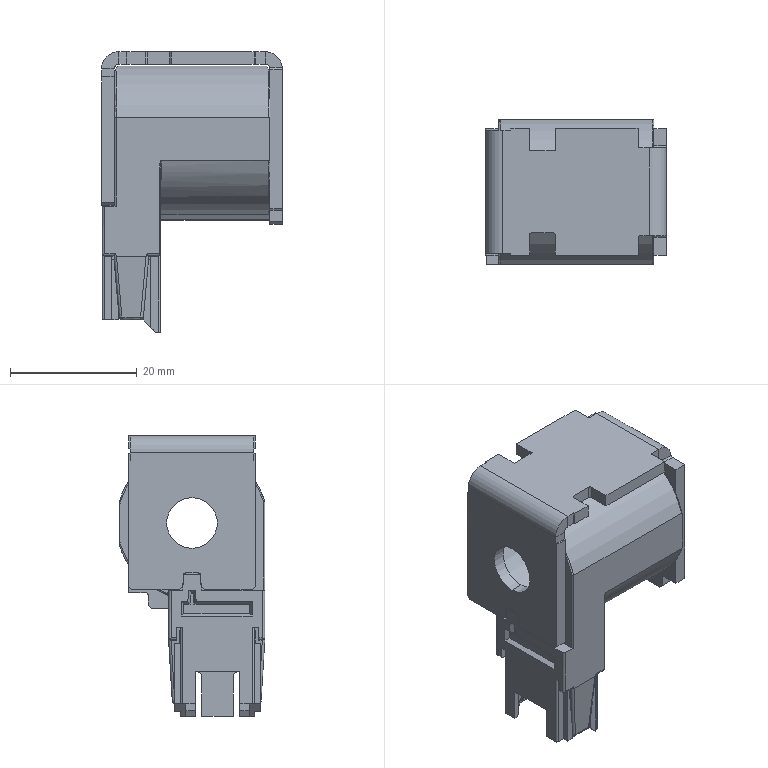Part | STEP file | ZXW735-L-95-01 | 1 solid | 515 faces | box 28.6 x 23 x 44.35 mm | volume 7211 mm3 | plane 335 | cylinder 116 | torus 35 | spline 18 | cone 6 | sphere 5 | commonest cylinder face diameters 0.4 x30 0.8 x20 0.6 x16 1 x10 20 x9 3 x4